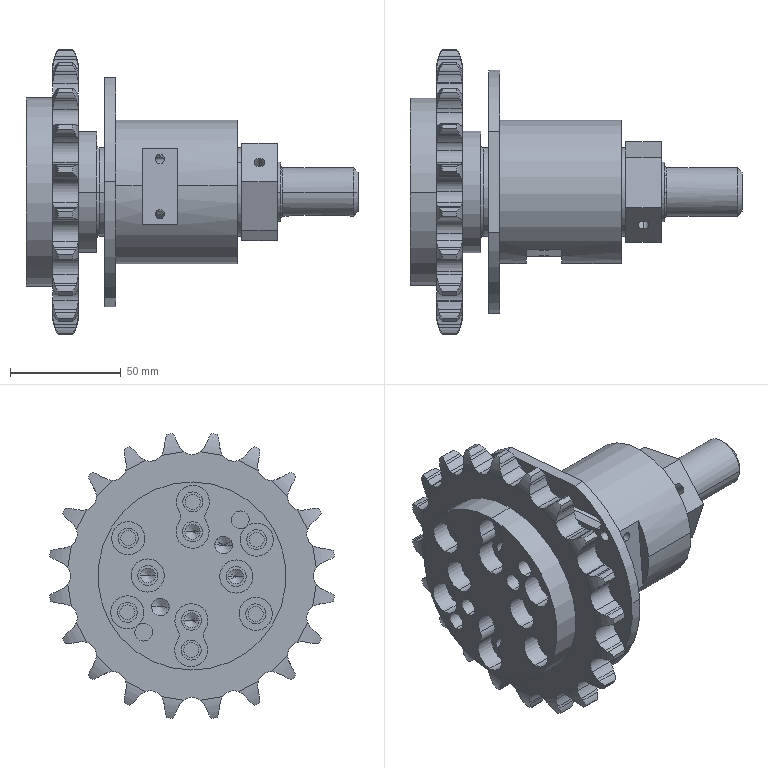Part | SolidWorks | features AEMSimFeature 1 | 7 solids | 799 faces | box 150 x 128.76 x 128.76 mm | volume 406242 mm3 | cylinder 317 | sphere 176 | plane 156 | torus 94 | spline 42 | cone 14 | commonest cylinder face diameters 17.336 x42 31.126 x42 12.07 x25 6.8 x20 9 x20 130 x20